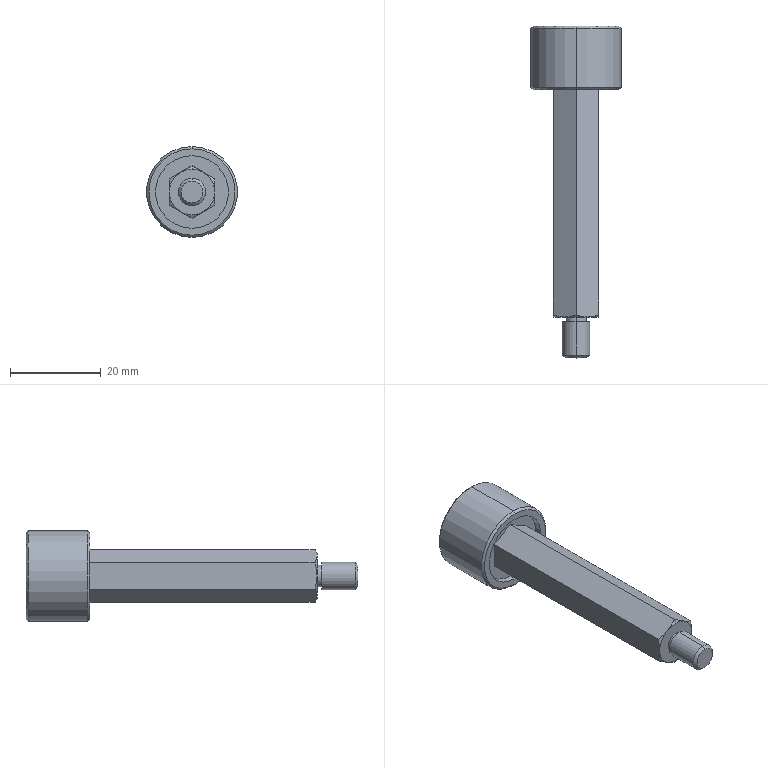Part | STEP file | 0243_010_RLLUP20-50 | 1 solid | 43 faces | box 20 x 73 x 20 mm | volume 8708 mm3 | plane 20 | cone 13 | cylinder 10 | commonest cylinder face diameters 4.65 x2 6 x2 12 x2 16 x2 20 x2